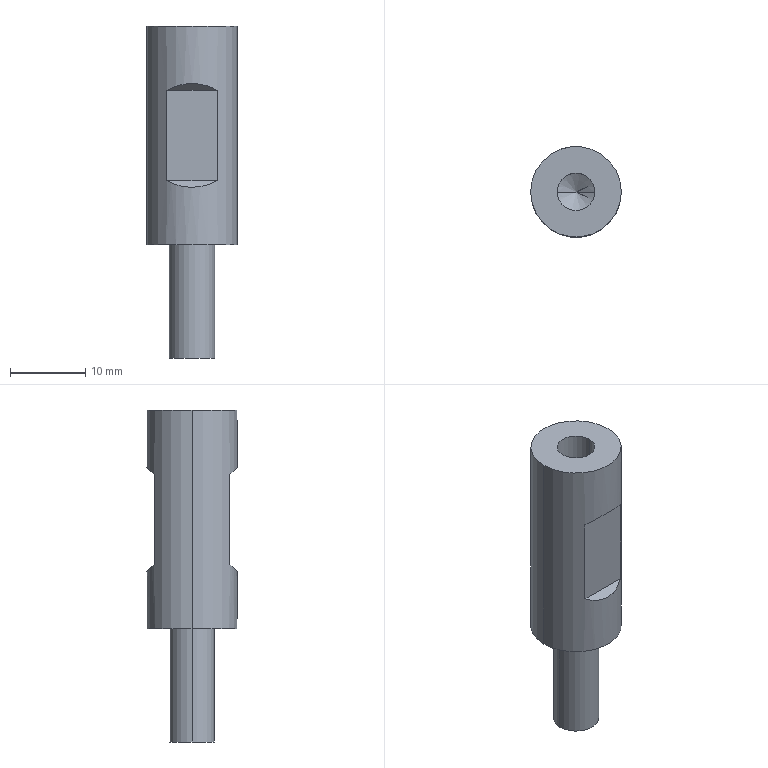Part | STEP file | MT-COMBO-119-S007_Default | 1 solid | 17 faces | box 12 x 12 x 44 mm | volume 3285 mm3 | plane 9 | cylinder 6 | cone 2 | commonest cylinder face diameters 5 x2 6 x2 12 x2
STEP:
#1=CARTESIAN_POINT('',(-2.5,0.,-15.));
#2=VERTEX_POINT('',#1);
#3=CARTESIAN_POINT('',(2.5,0.,-15.));
#4=VERTEX_POINT('',#3);
#5=CARTESIAN_POINT('',(0.,0.,-15.));
#6=DIRECTION('',(0.,0.,-1.));
#7=DIRECTION('',(-1.,0.,0.));
#8=AXIS2_PLACEMENT_3D('',#5,#6,#7);
#9=CIRCLE('',#8,2.5);
#10=EDGE_CURVE('',#2,#4,#9,.T.);
#11=ORIENTED_EDGE('',*,*,#10,.T.);
#12=CARTESIAN_POINT('',(2.5,0.,0.));
#13=VERTEX_POINT('',#12);
#14=CARTESIAN_POINT('',(2.5,0.,0.));
#15=DIRECTION('',(0.,0.,1.));
#16=VECTOR('',#15,1000.);
#17=LINE('',#14,#16);
#18=EDGE_CURVE('',#4,#13,#17,.T.);
#19=ORIENTED_EDGE('',*,*,#18,.T.);
#20=CARTESIAN_POINT('',(-2.5,0.,0.));
#21=VERTEX_POINT('',#20);
#22=CARTESIAN_POINT('',(0.,0.,0.));
#23=DIRECTION('',(0.,0.,-1.));
#24=DIRECTION('',(-1.,0.,0.));
#25=AXIS2_PLACEMENT_3D('',#22,#23,#24);
#26=CIRCLE('',#25,2.5);
#27=EDGE_CURVE('',#21,#13,#26,.T.);
#28=ORIENTED_EDGE('',*,*,#27,.F.);
#29=CARTESIAN_POINT('',(-2.5,0.,0.));
#30=DIRECTION('',(0.,0.,1.));
#31=VECTOR('',#30,1000.);
#32=LINE('',#29,#31);
#33=EDGE_CURVE('',#2,#21,#32,.T.);
#34=ORIENTED_EDGE('',*,*,#33,.F.);
#35=EDGE_LOOP('',(#11,#19,#28,#34));
#36=FACE_OUTER_BOUND('',#35,.T.);
#37=CARTESIAN_POINT('',(0.,0.,0.));
#38=DIRECTION('',(0.,0.,1.));
#39=DIRECTION('',(-1.,0.,0.));
#40=AXIS2_PLACEMENT_3D('',#37,#38,#39);
#41=CYLINDRICAL_SURFACE('',#40,2.5);
#42=ADVANCED_FACE('',(#36),#41,.F.);
#43=CARTESIAN_POINT('',(0.,0.,-16.502));
#44=VERTEX_POINT('',#43);
#45=CARTESIAN_POINT('',(-2.5,0.,-15.));
#46=DIRECTION('',(-0.8572,0.,0.515));
#47=VECTOR('',#46,1000.);
#48=LINE('',#45,#47);
#49=EDGE_CURVE('',#44,#2,#48,.T.);
#50=ORIENTED_EDGE('',*,*,#49,.F.);
#51=CARTESIAN_POINT('',(2.5,0.,-15.));
#52=DIRECTION('',(0.8572,0.,0.515));
#53=VECTOR('',#52,1000.);
#54=LINE('',#51,#53);
#55=EDGE_CURVE('',#44,#4,#54,.T.);
#56=ORIENTED_EDGE('',*,*,#55,.T.);
#57=ORIENTED_EDGE('',*,*,#10,.F.);
#58=EDGE_LOOP('',(#50,#56,#57));
#59=FACE_OUTER_BOUND('',#58,.T.);
#60=CARTESIAN_POINT('',(0.,0.,-15.));
#61=DIRECTION('',(0.,0.,1.));
#62=DIRECTION('',(-1.,0.,0.));
#63=AXIS2_PLACEMENT_3D('',#60,#61,#62);
#64=CONICAL_SURFACE('',#63,2.5,1.03);
#65=ADVANCED_FACE('',(#59),#64,.F.);
#66=CARTESIAN_POINT('',(-3.,0.,-44.));
#67=VERTEX_POINT('',#66);
#68=CARTESIAN_POINT('',(3.,0.,-44.));
#69=VERTEX_POINT('',#68);
#70=CARTESIAN_POINT('',(0.,0.,-44.));
#71=DIRECTION('',(0.,0.,1.));
#72=DIRECTION('',(1.,0.,0.));
#73=AXIS2_PLACEMENT_3D('',#70,#71,#72);
#74=CIRCLE('',#73,3.);
#75=EDGE_CURVE('',#67,#69,#74,.T.);
#76=ORIENTED_EDGE('',*,*,#75,.T.);
#77=CARTESIAN_POINT('',(3.,0.,-29.));
#78=VERTEX_POINT('',#77);
#79=CARTESIAN_POINT('',(3.,0.,-44.));
#80=DIRECTION('',(0.,0.,1.));
#81=VECTOR('',#80,1000.);
#82=LINE('',#79,#81);
#83=EDGE_CURVE('',#69,#78,#82,.T.);
#84=ORIENTED_EDGE('',*,*,#83,.T.);
#85=CARTESIAN_POINT('',(-3.,0.,-29.));
#86=VERTEX_POINT('',#85);
#87=CARTESIAN_POINT('',(0.,0.,-29.));
#88=DIRECTION('',(0.,0.,1.));
#89=DIRECTION('',(1.,0.,0.));
#90=AXIS2_PLACEMENT_3D('',#87,#88,#89);
#91=CIRCLE('',#90,3.);
#92=EDGE_CURVE('',#86,#78,#91,.T.);
#93=ORIENTED_EDGE('',*,*,#92,.F.);
#94=CARTESIAN_POINT('',(-3.,0.,-44.));
#95=DIRECTION('',(0.,0.,1.));
#96=VECTOR('',#95,1000.);
#97=LINE('',#94,#96);
#98=EDGE_CURVE('',#67,#86,#97,.T.);
#99=ORIENTED_EDGE('',*,*,#98,.F.);
#100=EDGE_LOOP('',(#76,#84,#93,#99));
#101=FACE_OUTER_BOUND('',#100,.T.);
#102=CARTESIAN_POINT('',(0.,0.,-44.));
#103=DIRECTION('',(0.,0.,1.));
#104=DIRECTION('',(-1.,0.,0.));
#105=AXIS2_PLACEMENT_3D('',#102,#103,#104);
#106=CYLINDRICAL_SURFACE('',#105,3.);
#107=ADVANCED_FACE('',(#101),#106,.T.);
#108=CARTESIAN_POINT('',(3.317,-5.,-20.5));
#109=VERTEX_POINT('',#108);
#110=CARTESIAN_POINT('',(-3.317,-5.,-20.5));
#111=VERTEX_POINT('',#110);
#112=CARTESIAN_POINT('',(3.317,-5.,-20.5));
#113=CARTESIAN_POINT('',(1.244,-6.375,-21.702));
#114=CARTESIAN_POINT('',(-1.244,-6.375,-21.702));
#115=CARTESIAN_POINT('',(-3.317,-5.,-20.5));
#116=(BOUNDED_CURVE()B_SPLINE_CURVE(3,(#112,#113,#114,#115),.UNSPECIFIED.,.F.,.T.)B_SPLINE_CURVE_WITH_KNOTS((4,4),(2.556,3.727),.UNSPECIFIED.)CURVE()GEOMETRIC_REPRESENTATION_ITEM()RATIONAL_B_SPLINE_CURVE((1.,0.8889,0.8889,1.))REPRESENTATION_ITEM(''));
#117=EDGE_CURVE('',#109,#111,#116,.T.);
#118=ORIENTED_EDGE('',*,*,#117,.T.);
#119=CARTESIAN_POINT('',(-3.317,-5.,-8.5));
#120=VERTEX_POINT('',#119);
#121=CARTESIAN_POINT('',(-3.317,-5.,-29.));
#122=DIRECTION('',(0.,0.,1.));
#123=VECTOR('',#122,1000.);
#124=LINE('',#121,#123);
#125=EDGE_CURVE('',#111,#120,#124,.T.);
#126=ORIENTED_EDGE('',*,*,#125,.T.);
#127=CARTESIAN_POINT('',(3.317,-5.,-8.5));
#128=VERTEX_POINT('',#127);
#129=CARTESIAN_POINT('',(-3.317,-5.,-8.5));
#130=CARTESIAN_POINT('',(-1.244,-6.375,-7.298));
#131=CARTESIAN_POINT('',(1.244,-6.375,-7.298));
#132=CARTESIAN_POINT('',(3.317,-5.,-8.5));
#133=(BOUNDED_CURVE()B_SPLINE_CURVE(3,(#129,#130,#131,#132),.UNSPECIFIED.,.F.,.T.)B_SPLINE_CURVE_WITH_KNOTS((4,4),(5.697,6.869),.UNSPECIFIED.)CURVE()GEOMETRIC_REPRESENTATION_ITEM()RATIONAL_B_SPLINE_CURVE((1.,0.8889,0.8889,1.))REPRESENTATION_ITEM(''));
#134=EDGE_CURVE('',#120,#128,#133,.T.);
#135=ORIENTED_EDGE('',*,*,#134,.T.);
#136=CARTESIAN_POINT('',(3.317,-5.,-29.));
#137=DIRECTION('',(0.,0.,-1.));
#138=VECTOR('',#137,1000.);
#139=LINE('',#136,#138);
#140=EDGE_CURVE('',#128,#109,#139,.T.);
#141=ORIENTED_EDGE('',*,*,#140,.T.);
#142=EDGE_LOOP('',(#118,#126,#135,#141));
#143=FACE_BOUND('',#142,.T.);
#144=CARTESIAN_POINT('',(-6.,0.,-29.));
#145=VERTEX_POINT('',#144);
#146=CARTESIAN_POINT('',(6.,0.,-29.));
#147=VERTEX_POINT('',#146);
#148=CARTESIAN_POINT('',(0.,0.,-29.));
#149=DIRECTION('',(0.,0.,1.));
#150=DIRECTION('',(1.,0.,0.));
#151=AXIS2_PLACEMENT_3D('',#148,#149,#150);
#152=CIRCLE('',#151,6.);
#153=EDGE_CURVE('',#145,#147,#152,.T.);
#154=ORIENTED_EDGE('',*,*,#153,.T.);
#155=CARTESIAN_POINT('',(6.,0.,0.));
#156=VERTEX_POINT('',#155);
#157=CARTESIAN_POINT('',(6.,0.,-29.));
#158=DIRECTION('',(0.,0.,1.));
#159=VECTOR('',#158,1000.);
#160=LINE('',#157,#159);
#161=EDGE_CURVE('',#147,#156,#160,.T.);
#162=ORIENTED_EDGE('',*,*,#161,.T.);
#163=CARTESIAN_POINT('',(-6.,0.,0.));
#164=VERTEX_POINT('',#163);
#165=CARTESIAN_POINT('',(0.,0.,0.));
#166=DIRECTION('',(0.,0.,1.));
#167=DIRECTION('',(1.,0.,0.));
#168=AXIS2_PLACEMENT_3D('',#165,#166,#167);
#169=CIRCLE('',#168,6.);
#170=EDGE_CURVE('',#164,#156,#169,.T.);
#171=ORIENTED_EDGE('',*,*,#170,.F.);
#172=CARTESIAN_POINT('',(-6.,0.,-29.));
#173=DIRECTION('',(0.,0.,1.));
#174=VECTOR('',#173,1000.);
#175=LINE('',#172,#174);
#176=EDGE_CURVE('',#145,#164,#175,.T.);
#177=ORIENTED_EDGE('',*,*,#176,.F.);
#178=EDGE_LOOP('',(#154,#162,#171,#177));
#179=FACE_OUTER_BOUND('',#178,.T.);
#180=CARTESIAN_POINT('',(0.,0.,-29.));
#181=DIRECTION('',(0.,0.,1.));
#182=DIRECTION('',(-1.,0.,0.));
#183=AXIS2_PLACEMENT_3D('',#180,#181,#182);
#184=CYLINDRICAL_SURFACE('',#183,6.);
#185=ADVANCED_FACE('',(#143,#179),#184,.T.);
#186=ORIENTED_EDGE('',*,*,#161,.F.);
#187=CARTESIAN_POINT('',(0.,0.,-29.));
#188=DIRECTION('',(0.,0.,1.));
#189=DIRECTION('',(1.,0.,0.));
#190=AXIS2_PLACEMENT_3D('',#187,#188,#189);
#191=CIRCLE('',#190,6.);
#192=EDGE_CURVE('',#147,#145,#191,.T.);
#193=ORIENTED_EDGE('',*,*,#192,.T.);
#194=ORIENTED_EDGE('',*,*,#176,.T.);
#195=CARTESIAN_POINT('',(0.,0.,0.));
#196=DIRECTION('',(0.,0.,1.));
#197=DIRECTION('',(1.,0.,0.));
#198=AXIS2_PLACEMENT_3D('',#195,#196,#197);
#199=CIRCLE('',#198,6.);
#200=EDGE_CURVE('',#156,#164,#199,.T.);
#201=ORIENTED_EDGE('',*,*,#200,.F.);
#202=EDGE_LOOP('',(#186,#193,#194,#201));
#203=FACE_OUTER_BOUND('',#202,.T.);
#204=CARTESIAN_POINT('',(-3.317,5.,-20.5));
#205=VERTEX_POINT('',#204);
#206=CARTESIAN_POINT('',(-3.317,5.,-8.5));
#207=VERTEX_POINT('',#206);
#208=CARTESIAN_POINT('',(-3.317,5.,-29.));
#209=DIRECTION('',(0.,0.,1.));
#210=VECTOR('',#209,1000.);
#211=LINE('',#208,#210);
#212=EDGE_CURVE('',#205,#207,#211,.T.);
#213=ORIENTED_EDGE('',*,*,#212,.F.);
#214=CARTESIAN_POINT('',(3.317,5.,-20.5));
#215=VERTEX_POINT('',#214);
#216=CARTESIAN_POINT('',(3.317,5.,-20.5));
#217=CARTESIAN_POINT('',(1.244,6.375,-21.702));
#218=CARTESIAN_POINT('',(-1.244,6.375,-21.702));
#219=CARTESIAN_POINT('',(-3.317,5.,-20.5));
#220=(BOUNDED_CURVE()B_SPLINE_CURVE(3,(#216,#217,#218,#219),.UNSPECIFIED.,.F.,.T.)B_SPLINE_CURVE_WITH_KNOTS((4,4),(2.556,3.727),.UNSPECIFIED.)CURVE()GEOMETRIC_REPRESENTATION_ITEM()RATIONAL_B_SPLINE_CURVE((1.,0.8889,0.8889,1.))REPRESENTATION_ITEM(''));
#221=EDGE_CURVE('',#215,#205,#220,.T.);
#222=ORIENTED_EDGE('',*,*,#221,.F.);
#223=CARTESIAN_POINT('',(3.317,5.,-8.5));
#224=VERTEX_POINT('',#223);
#225=CARTESIAN_POINT('',(3.317,5.,-29.));
#226=DIRECTION('',(0.,0.,-1.));
#227=VECTOR('',#226,1000.);
#228=LINE('',#225,#227);
#229=EDGE_CURVE('',#224,#215,#228,.T.);
#230=ORIENTED_EDGE('',*,*,#229,.F.);
#231=CARTESIAN_POINT('',(-3.317,5.,-8.5));
#232=CARTESIAN_POINT('',(-1.244,6.375,-7.298));
#233=CARTESIAN_POINT('',(1.244,6.375,-7.298));
#234=CARTESIAN_POINT('',(3.317,5.,-8.5));
#235=(BOUNDED_CURVE()B_SPLINE_CURVE(3,(#231,#232,#233,#234),.UNSPECIFIED.,.F.,.T.)B_SPLINE_CURVE_WITH_KNOTS((4,4),(5.697,6.869),.UNSPECIFIED.)CURVE()GEOMETRIC_REPRESENTATION_ITEM()RATIONAL_B_SPLINE_CURVE((1.,0.8889,0.8889,1.))REPRESENTATION_ITEM(''));
#236=EDGE_CURVE('',#207,#224,#235,.T.);
#237=ORIENTED_EDGE('',*,*,#236,.F.);
#238=EDGE_LOOP('',(#213,#222,#230,#237));
#239=FACE_BOUND('',#238,.T.);
#240=CARTESIAN_POINT('',(0.,0.,-29.));
#241=DIRECTION('',(0.,0.,1.));
#242=DIRECTION('',(-1.,0.,0.));
#243=AXIS2_PLACEMENT_3D('',#240,#241,#242);
#244=CYLINDRICAL_SURFACE('',#243,6.);
#245=ADVANCED_FACE('',(#203,#239),#244,.T.);
#246=ORIENTED_EDGE('',*,*,#153,.F.);
#247=ORIENTED_EDGE('',*,*,#192,.F.);
#248=EDGE_LOOP('',(#246,#247));
#249=FACE_OUTER_BOUND('',#248,.T.);
#250=ORIENTED_EDGE('',*,*,#92,.T.);
#251=CARTESIAN_POINT('',(0.,0.,-29.));
#252=DIRECTION('',(0.,0.,1.));
#253=DIRECTION('',(1.,0.,0.));
#254=AXIS2_PLACEMENT_3D('',#251,#252,#253);
#255=CIRCLE('',#254,3.);
#256=EDGE_CURVE('',#78,#86,#255,.T.);
#257=ORIENTED_EDGE('',*,*,#256,.T.);
#258=EDGE_LOOP('',(#250,#257));
#259=FACE_BOUND('',#258,.T.);
#260=CARTESIAN_POINT('',(0.,0.,-29.));
#261=DIRECTION('',(0.,0.,-1.));
#262=DIRECTION('',(1.,0.,0.));
#263=AXIS2_PLACEMENT_3D('',#260,#261,#262);
#264=PLANE('',#263);
#265=ADVANCED_FACE('',(#249,#259),#264,.T.);
#266=ORIENTED_EDGE('',*,*,#27,.T.);
#267=CARTESIAN_POINT('',(0.,0.,0.));
#268=DIRECTION('',(0.,0.,-1.));
#269=DIRECTION('',(-1.,0.,0.));
#270=AXIS2_PLACEMENT_3D('',#267,#268,#269);
#271=CIRCLE('',#270,2.5);
#272=EDGE_CURVE('',#13,#21,#271,.T.);
#273=ORIENTED_EDGE('',*,*,#272,.T.);
#274=EDGE_LOOP('',(#266,#273));
#275=FACE_BOUND('',#274,.T.);
#276=ORIENTED_EDGE('',*,*,#170,.T.);
#277=ORIENTED_EDGE('',*,*,#200,.T.);
#278=EDGE_LOOP('',(#276,#277));
#279=FACE_OUTER_BOUND('',#278,.T.);
#280=CARTESIAN_POINT('',(0.,0.,0.));
#281=DIRECTION('',(0.,0.,-1.));
#282=DIRECTION('',(1.,0.,0.));
#283=AXIS2_PLACEMENT_3D('',#280,#281,#282);
#284=PLANE('',#283);
#285=ADVANCED_FACE('',(#275,#279),#284,.F.);
#286=ORIENTED_EDGE('',*,*,#83,.F.);
#287=CARTESIAN_POINT('',(0.,0.,-44.));
#288=DIRECTION('',(0.,0.,1.));
#289=DIRECTION('',(1.,0.,0.));
#290=AXIS2_PLACEMENT_3D('',#287,#288,#289);
#291=CIRCLE('',#290,3.);
#292=EDGE_CURVE('',#69,#67,#291,.T.);
#293=ORIENTED_EDGE('',*,*,#292,.T.);
#294=ORIENTED_EDGE('',*,*,#98,.T.);
#295=ORIENTED_EDGE('',*,*,#256,.F.);
#296=EDGE_LOOP('',(#286,#293,#294,#295));
#297=FACE_OUTER_BOUND('',#296,.T.);
#298=CARTESIAN_POINT('',(0.,0.,-44.));
#299=DIRECTION('',(0.,0.,1.));
#300=DIRECTION('',(-1.,0.,0.));
#301=AXIS2_PLACEMENT_3D('',#298,#299,#300);
#302=CYLINDRICAL_SURFACE('',#301,3.);
#303=ADVANCED_FACE('',(#297),#302,.T.);
#304=ORIENTED_EDGE('',*,*,#75,.F.);
#305=ORIENTED_EDGE('',*,*,#292,.F.);
#306=EDGE_LOOP('',(#304,#305));
#307=FACE_OUTER_BOUND('',#306,.T.);
#308=CARTESIAN_POINT('',(0.,0.,-44.));
#309=DIRECTION('',(0.,0.,-1.));
#310=DIRECTION('',(1.,0.,0.));
#311=AXIS2_PLACEMENT_3D('',#308,#309,#310);
#312=PLANE('',#311);
#313=ADVANCED_FACE('',(#307),#312,.T.);
#314=CARTESIAN_POINT('',(-7.5,5.,-8.5));
#315=DIRECTION('',(1.,0.,0.));
#316=VECTOR('',#315,1000.);
#317=LINE('',#314,#316);
#318=EDGE_CURVE('',#207,#224,#317,.T.);
#319=ORIENTED_EDGE('',*,*,#318,.F.);
#320=ORIENTED_EDGE('',*,*,#236,.T.);
#321=EDGE_LOOP('',(#319,#320));
#322=FACE_OUTER_BOUND('',#321,.T.);
#323=CARTESIAN_POINT('',(-7.5,5.,-8.5));
#324=DIRECTION('',(0.,-0.6581,0.753));
#325=DIRECTION('',(0.,0.753,0.6581));
#326=AXIS2_PLACEMENT_3D('',#323,#324,#325);
#327=PLANE('',#326);
#328=ADVANCED_FACE('',(#322),#327,.F.);
#329=CARTESIAN_POINT('',(-7.5,5.,-20.5));
#330=DIRECTION('',(1.,0.,0.));
#331=VECTOR('',#330,1000.);
#332=LINE('',#329,#331);
#333=EDGE_CURVE('',#205,#215,#332,.T.);
#334=ORIENTED_EDGE('',*,*,#333,.F.);
#335=ORIENTED_EDGE('',*,*,#212,.T.);
#336=ORIENTED_EDGE('',*,*,#318,.T.);
#337=ORIENTED_EDGE('',*,*,#229,.T.);
#338=EDGE_LOOP('',(#334,#335,#336,#337));
#339=FACE_OUTER_BOUND('',#338,.T.);
#340=CARTESIAN_POINT('',(-7.5,5.,-20.5));
#341=DIRECTION('',(0.,-1.,0.));
#342=DIRECTION('',(0.,0.,1.));
#343=AXIS2_PLACEMENT_3D('',#340,#341,#342);
#344=PLANE('',#343);
#345=ADVANCED_FACE('',(#339),#344,.F.);
#346=ORIENTED_EDGE('',*,*,#333,.T.);
#347=ORIENTED_EDGE('',*,*,#221,.T.);
#348=EDGE_LOOP('',(#346,#347));
#349=FACE_OUTER_BOUND('',#348,.T.);
#350=CARTESIAN_POINT('',(-7.5,9.577,-24.5));
#351=DIRECTION('',(0.,-0.6581,-0.753));
#352=DIRECTION('',(0.,-0.753,0.6581));
#353=AXIS2_PLACEMENT_3D('',#350,#351,#352);
#354=PLANE('',#353);
#355=ADVANCED_FACE('',(#349),#354,.F.);
#356=ORIENTED_EDGE('',*,*,#117,.F.);
#357=CARTESIAN_POINT('',(-7.5,-5.,-20.5));
#358=DIRECTION('',(1.,0.,0.));
#359=VECTOR('',#358,1000.);
#360=LINE('',#357,#359);
#361=EDGE_CURVE('',#111,#109,#360,.T.);
#362=ORIENTED_EDGE('',*,*,#361,.F.);
#363=EDGE_LOOP('',(#356,#362));
#364=FACE_OUTER_BOUND('',#363,.T.);
#365=CARTESIAN_POINT('',(-7.5,-9.577,-24.5));
#366=DIRECTION('',(0.,-0.6581,0.753));
#367=DIRECTION('',(0.,0.753,0.6581));
#368=AXIS2_PLACEMENT_3D('',#365,#366,#367);
#369=PLANE('',#368);
#370=ADVANCED_FACE('',(#364),#369,.T.);
#371=ORIENTED_EDGE('',*,*,#125,.F.);
#372=ORIENTED_EDGE('',*,*,#361,.T.);
#373=ORIENTED_EDGE('',*,*,#140,.F.);
#374=CARTESIAN_POINT('',(-7.5,-5.,-8.5));
#375=DIRECTION('',(1.,0.,0.));
#376=VECTOR('',#375,1000.);
#377=LINE('',#374,#376);
#378=EDGE_CURVE('',#120,#128,#377,.T.);
#379=ORIENTED_EDGE('',*,*,#378,.F.);
#380=EDGE_LOOP('',(#371,#372,#373,#379));
#381=FACE_OUTER_BOUND('',#380,.T.);
#382=CARTESIAN_POINT('',(-7.5,-5.,-20.5));
#383=DIRECTION('',(0.,-1.,0.));
#384=DIRECTION('',(0.,0.,1.));
#385=AXIS2_PLACEMENT_3D('',#382,#383,#384);
#386=PLANE('',#385);
#387=ADVANCED_FACE('',(#381),#386,.T.);
#388=ORIENTED_EDGE('',*,*,#134,.F.);
#389=ORIENTED_EDGE('',*,*,#378,.T.);
#390=EDGE_LOOP('',(#388,#389));
#391=FACE_OUTER_BOUND('',#390,.T.);
#392=CARTESIAN_POINT('',(-7.5,-5.,-8.5));
#393=DIRECTION('',(0.,-0.6581,-0.753));
#394=DIRECTION('',(0.,-0.753,0.6581));
#395=AXIS2_PLACEMENT_3D('',#392,#393,#394);
#396=PLANE('',#395);
#397=ADVANCED_FACE('',(#391),#396,.T.);
#398=ORIENTED_EDGE('',*,*,#55,.F.);
#399=ORIENTED_EDGE('',*,*,#49,.T.);
#400=CARTESIAN_POINT('',(0.,0.,-15.));
#401=DIRECTION('',(0.,0.,-1.));
#402=DIRECTION('',(-1.,0.,0.));
#403=AXIS2_PLACEMENT_3D('',#400,#401,#402);
#404=CIRCLE('',#403,2.5);
#405=EDGE_CURVE('',#4,#2,#404,.T.);
#406=ORIENTED_EDGE('',*,*,#405,.F.);
#407=EDGE_LOOP('',(#398,#399,#406));
#408=FACE_OUTER_BOUND('',#407,.T.);
#409=CARTESIAN_POINT('',(0.,0.,-15.));
#410=DIRECTION('',(0.,0.,1.));
#411=DIRECTION('',(-1.,0.,0.));
#412=AXIS2_PLACEMENT_3D('',#409,#410,#411);
#413=CONICAL_SURFACE('',#412,2.5,1.03);
#414=ADVANCED_FACE('',(#408),#413,.F.);
#415=ORIENTED_EDGE('',*,*,#18,.F.);
#416=ORIENTED_EDGE('',*,*,#405,.T.);
#417=ORIENTED_EDGE('',*,*,#33,.T.);
#418=ORIENTED_EDGE('',*,*,#272,.F.);
#419=EDGE_LOOP('',(#415,#416,#417,#418));
#420=FACE_OUTER_BOUND('',#419,.T.);
#421=CARTESIAN_POINT('',(0.,0.,0.));
#422=DIRECTION('',(0.,0.,1.));
#423=DIRECTION('',(-1.,0.,0.));
#424=AXIS2_PLACEMENT_3D('',#421,#422,#423);
#425=CYLINDRICAL_SURFACE('',#424,2.5);
#426=ADVANCED_FACE('',(#420),#425,.F.);
#427=CLOSED_SHELL('',(#42,#65,#107,#185,#245,#265,#285,#303,#313,#328,#345,#355,#370,#387,#397,#414,#426));
#428=MANIFOLD_SOLID_BREP('',#427);
#429=CARTESIAN_POINT('',(0.,0.,0.));
#430=DIRECTION('',(0.,0.,1.));
#431=DIRECTION('',(1.,0.,0.));
#432=AXIS2_PLACEMENT_3D('',#429,#430,#431);
#433=(LENGTH_UNIT()NAMED_UNIT(*)SI_UNIT(.MILLI.,.METRE.));
#434=UNCERTAINTY_MEASURE_WITH_UNIT(LENGTH_MEASURE(0.00001),#433,'','');
#435=(NAMED_UNIT(*)PLANE_ANGLE_UNIT()SI_UNIT($,.RADIAN.));
#436=(NAMED_UNIT(*)SI_UNIT($,.STERADIAN.)SOLID_ANGLE_UNIT());
#437=(GEOMETRIC_REPRESENTATION_CONTEXT(3)GLOBAL_UNCERTAINTY_ASSIGNED_CONTEXT((#434))GLOBAL_UNIT_ASSIGNED_CONTEXT((#433,#435,#436))REPRESENTATION_CONTEXT('',''));
#438=ADVANCED_BREP_SHAPE_REPRESENTATION('',(#428,#432),#437);